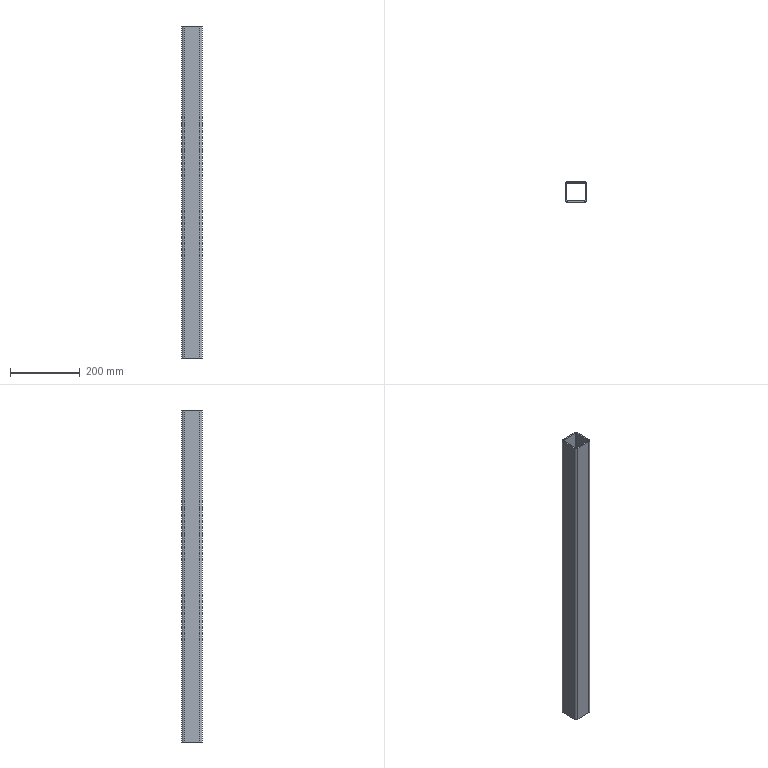Part | SolidWorks | features ICE 1, LibraryFeature 1 | 1 solid | 18 faces | box 60 x 60 x 950 mm | volume 812057 mm3 | plane 10 | cylinder 8 | commonest cylinder face diameters 8 x4 16 x4
STEP:
#1=CARTESIAN_POINT('',(22.,30.,0.));
#2=VERTEX_POINT('',#1);
#3=CARTESIAN_POINT('',(-22.,30.,0.));
#4=VERTEX_POINT('',#3);
#5=CARTESIAN_POINT('',(0.,30.,0.));
#6=DIRECTION('',(-1.,0.,0.));
#7=VECTOR('',#6,1000.);
#8=LINE('',#5,#7);
#9=EDGE_CURVE('',#2,#4,#8,.T.);
#10=ORIENTED_EDGE('',*,*,#9,.T.);
#11=CARTESIAN_POINT('',(-22.,30.,950.));
#12=VERTEX_POINT('',#11);
#13=CARTESIAN_POINT('',(-22.,30.,950.));
#14=DIRECTION('',(0.,0.,-1.));
#15=VECTOR('',#14,1000.);
#16=LINE('',#13,#15);
#17=EDGE_CURVE('',#12,#4,#16,.T.);
#18=ORIENTED_EDGE('',*,*,#17,.F.);
#19=CARTESIAN_POINT('',(22.,30.,950.));
#20=VERTEX_POINT('',#19);
#21=CARTESIAN_POINT('',(0.,30.,950.));
#22=DIRECTION('',(-1.,0.,0.));
#23=VECTOR('',#22,1000.);
#24=LINE('',#21,#23);
#25=EDGE_CURVE('',#20,#12,#24,.T.);
#26=ORIENTED_EDGE('',*,*,#25,.F.);
#27=CARTESIAN_POINT('',(22.,30.,950.));
#28=DIRECTION('',(0.,0.,-1.));
#29=VECTOR('',#28,1000.);
#30=LINE('',#27,#29);
#31=EDGE_CURVE('',#20,#2,#30,.T.);
#32=ORIENTED_EDGE('',*,*,#31,.T.);
#33=EDGE_LOOP('',(#10,#18,#26,#32));
#34=FACE_OUTER_BOUND('',#33,.T.);
#35=CARTESIAN_POINT('',(0.,30.,950.));
#36=DIRECTION('',(0.,-1.,0.));
#37=DIRECTION('',(0.,0.,-1.));
#38=AXIS2_PLACEMENT_3D('',#35,#36,#37);
#39=PLANE('',#38);
#40=ADVANCED_FACE('',(#34),#39,.F.);
#41=CARTESIAN_POINT('',(-30.,22.,0.));
#42=VERTEX_POINT('',#41);
#43=CARTESIAN_POINT('',(-22.,22.,0.));
#44=DIRECTION('',(0.,0.,1.));
#45=DIRECTION('',(1.,0.,0.));
#46=AXIS2_PLACEMENT_3D('',#43,#44,#45);
#47=CIRCLE('',#46,8.);
#48=EDGE_CURVE('',#4,#42,#47,.T.);
#49=ORIENTED_EDGE('',*,*,#48,.T.);
#50=CARTESIAN_POINT('',(-30.,22.,950.));
#51=VERTEX_POINT('',#50);
#52=CARTESIAN_POINT('',(-30.,22.,950.));
#53=DIRECTION('',(0.,0.,-1.));
#54=VECTOR('',#53,1000.);
#55=LINE('',#52,#54);
#56=EDGE_CURVE('',#51,#42,#55,.T.);
#57=ORIENTED_EDGE('',*,*,#56,.F.);
#58=CARTESIAN_POINT('',(-22.,22.,950.));
#59=DIRECTION('',(0.,0.,1.));
#60=DIRECTION('',(1.,0.,0.));
#61=AXIS2_PLACEMENT_3D('',#58,#59,#60);
#62=CIRCLE('',#61,8.);
#63=EDGE_CURVE('',#12,#51,#62,.T.);
#64=ORIENTED_EDGE('',*,*,#63,.F.);
#65=ORIENTED_EDGE('',*,*,#17,.T.);
#66=EDGE_LOOP('',(#49,#57,#64,#65));
#67=FACE_OUTER_BOUND('',#66,.T.);
#68=CARTESIAN_POINT('',(-22.,22.,950.));
#69=DIRECTION('',(0.,0.,-1.));
#70=DIRECTION('',(-1.,0.,0.));
#71=AXIS2_PLACEMENT_3D('',#68,#69,#70);
#72=CYLINDRICAL_SURFACE('',#71,8.);
#73=ADVANCED_FACE('',(#67),#72,.T.);
#74=CARTESIAN_POINT('',(-30.,-22.,0.));
#75=VERTEX_POINT('',#74);
#76=CARTESIAN_POINT('',(-30.,0.,0.));
#77=DIRECTION('',(0.,1.,0.));
#78=VECTOR('',#77,1000.);
#79=LINE('',#76,#78);
#80=EDGE_CURVE('',#75,#42,#79,.T.);
#81=ORIENTED_EDGE('',*,*,#80,.F.);
#82=CARTESIAN_POINT('',(-30.,-22.,950.));
#83=VERTEX_POINT('',#82);
#84=CARTESIAN_POINT('',(-30.,-22.,950.));
#85=DIRECTION('',(0.,0.,-1.));
#86=VECTOR('',#85,1000.);
#87=LINE('',#84,#86);
#88=EDGE_CURVE('',#83,#75,#87,.T.);
#89=ORIENTED_EDGE('',*,*,#88,.F.);
#90=CARTESIAN_POINT('',(-30.,0.,950.));
#91=DIRECTION('',(0.,1.,0.));
#92=VECTOR('',#91,1000.);
#93=LINE('',#90,#92);
#94=EDGE_CURVE('',#83,#51,#93,.T.);
#95=ORIENTED_EDGE('',*,*,#94,.T.);
#96=ORIENTED_EDGE('',*,*,#56,.T.);
#97=EDGE_LOOP('',(#81,#89,#95,#96));
#98=FACE_OUTER_BOUND('',#97,.T.);
#99=CARTESIAN_POINT('',(-30.,0.,950.));
#100=DIRECTION('',(-1.,0.,0.));
#101=DIRECTION('',(0.,0.,1.));
#102=AXIS2_PLACEMENT_3D('',#99,#100,#101);
#103=PLANE('',#102);
#104=ADVANCED_FACE('',(#98),#103,.T.);
#105=CARTESIAN_POINT('',(-22.,-30.,0.));
#106=VERTEX_POINT('',#105);
#107=CARTESIAN_POINT('',(-22.,-22.,0.));
#108=DIRECTION('',(0.,0.,1.));
#109=DIRECTION('',(1.,0.,0.));
#110=AXIS2_PLACEMENT_3D('',#107,#108,#109);
#111=CIRCLE('',#110,8.);
#112=EDGE_CURVE('',#75,#106,#111,.T.);
#113=ORIENTED_EDGE('',*,*,#112,.T.);
#114=CARTESIAN_POINT('',(-22.,-30.,950.));
#115=VERTEX_POINT('',#114);
#116=CARTESIAN_POINT('',(-22.,-30.,950.));
#117=DIRECTION('',(0.,0.,-1.));
#118=VECTOR('',#117,1000.);
#119=LINE('',#116,#118);
#120=EDGE_CURVE('',#115,#106,#119,.T.);
#121=ORIENTED_EDGE('',*,*,#120,.F.);
#122=CARTESIAN_POINT('',(-22.,-22.,950.));
#123=DIRECTION('',(0.,0.,1.));
#124=DIRECTION('',(1.,0.,0.));
#125=AXIS2_PLACEMENT_3D('',#122,#123,#124);
#126=CIRCLE('',#125,8.);
#127=EDGE_CURVE('',#83,#115,#126,.T.);
#128=ORIENTED_EDGE('',*,*,#127,.F.);
#129=ORIENTED_EDGE('',*,*,#88,.T.);
#130=EDGE_LOOP('',(#113,#121,#128,#129));
#131=FACE_OUTER_BOUND('',#130,.T.);
#132=CARTESIAN_POINT('',(-22.,-22.,950.));
#133=DIRECTION('',(0.,0.,-1.));
#134=DIRECTION('',(-1.,0.,0.));
#135=AXIS2_PLACEMENT_3D('',#132,#133,#134);
#136=CYLINDRICAL_SURFACE('',#135,8.);
#137=ADVANCED_FACE('',(#131),#136,.T.);
#138=CARTESIAN_POINT('',(22.,-30.,0.));
#139=VERTEX_POINT('',#138);
#140=CARTESIAN_POINT('',(0.,-30.,0.));
#141=DIRECTION('',(1.,0.,0.));
#142=VECTOR('',#141,1000.);
#143=LINE('',#140,#142);
#144=EDGE_CURVE('',#106,#139,#143,.T.);
#145=ORIENTED_EDGE('',*,*,#144,.T.);
#146=CARTESIAN_POINT('',(22.,-30.,950.));
#147=VERTEX_POINT('',#146);
#148=CARTESIAN_POINT('',(22.,-30.,950.));
#149=DIRECTION('',(0.,0.,-1.));
#150=VECTOR('',#149,1000.);
#151=LINE('',#148,#150);
#152=EDGE_CURVE('',#147,#139,#151,.T.);
#153=ORIENTED_EDGE('',*,*,#152,.F.);
#154=CARTESIAN_POINT('',(0.,-30.,950.));
#155=DIRECTION('',(1.,0.,0.));
#156=VECTOR('',#155,1000.);
#157=LINE('',#154,#156);
#158=EDGE_CURVE('',#115,#147,#157,.T.);
#159=ORIENTED_EDGE('',*,*,#158,.F.);
#160=ORIENTED_EDGE('',*,*,#120,.T.);
#161=EDGE_LOOP('',(#145,#153,#159,#160));
#162=FACE_OUTER_BOUND('',#161,.T.);
#163=CARTESIAN_POINT('',(0.,-30.,950.));
#164=DIRECTION('',(0.,1.,0.));
#165=DIRECTION('',(0.,0.,1.));
#166=AXIS2_PLACEMENT_3D('',#163,#164,#165);
#167=PLANE('',#166);
#168=ADVANCED_FACE('',(#162),#167,.F.);
#169=CARTESIAN_POINT('',(30.,-22.,0.));
#170=VERTEX_POINT('',#169);
#171=CARTESIAN_POINT('',(22.,-22.,0.));
#172=DIRECTION('',(0.,0.,1.));
#173=DIRECTION('',(1.,0.,0.));
#174=AXIS2_PLACEMENT_3D('',#171,#172,#173);
#175=CIRCLE('',#174,8.);
#176=EDGE_CURVE('',#139,#170,#175,.T.);
#177=ORIENTED_EDGE('',*,*,#176,.T.);
#178=CARTESIAN_POINT('',(30.,-22.,950.));
#179=VERTEX_POINT('',#178);
#180=CARTESIAN_POINT('',(30.,-22.,950.));
#181=DIRECTION('',(0.,0.,-1.));
#182=VECTOR('',#181,1000.);
#183=LINE('',#180,#182);
#184=EDGE_CURVE('',#179,#170,#183,.T.);
#185=ORIENTED_EDGE('',*,*,#184,.F.);
#186=CARTESIAN_POINT('',(22.,-22.,950.));
#187=DIRECTION('',(0.,0.,1.));
#188=DIRECTION('',(1.,0.,0.));
#189=AXIS2_PLACEMENT_3D('',#186,#187,#188);
#190=CIRCLE('',#189,8.);
#191=EDGE_CURVE('',#147,#179,#190,.T.);
#192=ORIENTED_EDGE('',*,*,#191,.F.);
#193=ORIENTED_EDGE('',*,*,#152,.T.);
#194=EDGE_LOOP('',(#177,#185,#192,#193));
#195=FACE_OUTER_BOUND('',#194,.T.);
#196=CARTESIAN_POINT('',(22.,-22.,950.));
#197=DIRECTION('',(0.,0.,-1.));
#198=DIRECTION('',(-1.,0.,0.));
#199=AXIS2_PLACEMENT_3D('',#196,#197,#198);
#200=CYLINDRICAL_SURFACE('',#199,8.);
#201=ADVANCED_FACE('',(#195),#200,.T.);
#202=CARTESIAN_POINT('',(30.,22.,0.));
#203=VERTEX_POINT('',#202);
#204=CARTESIAN_POINT('',(30.,0.,0.));
#205=DIRECTION('',(0.,-1.,0.));
#206=VECTOR('',#205,1000.);
#207=LINE('',#204,#206);
#208=EDGE_CURVE('',#203,#170,#207,.T.);
#209=ORIENTED_EDGE('',*,*,#208,.F.);
#210=CARTESIAN_POINT('',(30.,22.,950.));
#211=VERTEX_POINT('',#210);
#212=CARTESIAN_POINT('',(30.,22.,950.));
#213=DIRECTION('',(0.,0.,-1.));
#214=VECTOR('',#213,1000.);
#215=LINE('',#212,#214);
#216=EDGE_CURVE('',#211,#203,#215,.T.);
#217=ORIENTED_EDGE('',*,*,#216,.F.);
#218=CARTESIAN_POINT('',(30.,0.,950.));
#219=DIRECTION('',(0.,-1.,0.));
#220=VECTOR('',#219,1000.);
#221=LINE('',#218,#220);
#222=EDGE_CURVE('',#211,#179,#221,.T.);
#223=ORIENTED_EDGE('',*,*,#222,.T.);
#224=ORIENTED_EDGE('',*,*,#184,.T.);
#225=EDGE_LOOP('',(#209,#217,#223,#224));
#226=FACE_OUTER_BOUND('',#225,.T.);
#227=CARTESIAN_POINT('',(30.,0.,950.));
#228=DIRECTION('',(1.,0.,0.));
#229=DIRECTION('',(0.,0.,-1.));
#230=AXIS2_PLACEMENT_3D('',#227,#228,#229);
#231=PLANE('',#230);
#232=ADVANCED_FACE('',(#226),#231,.T.);
#233=CARTESIAN_POINT('',(-26.,-22.,0.));
#234=VERTEX_POINT('',#233);
#235=CARTESIAN_POINT('',(-22.,-26.,0.));
#236=VERTEX_POINT('',#235);
#237=CARTESIAN_POINT('',(-22.,-22.,0.));
#238=DIRECTION('',(0.,0.,1.));
#239=DIRECTION('',(1.,0.,0.));
#240=AXIS2_PLACEMENT_3D('',#237,#238,#239);
#241=CIRCLE('',#240,4.);
#242=EDGE_CURVE('',#234,#236,#241,.T.);
#243=ORIENTED_EDGE('',*,*,#242,.F.);
#244=CARTESIAN_POINT('',(-26.,-22.,950.));
#245=VERTEX_POINT('',#244);
#246=CARTESIAN_POINT('',(-26.,-22.,950.));
#247=DIRECTION('',(0.,0.,-1.));
#248=VECTOR('',#247,1000.);
#249=LINE('',#246,#248);
#250=EDGE_CURVE('',#245,#234,#249,.T.);
#251=ORIENTED_EDGE('',*,*,#250,.F.);
#252=CARTESIAN_POINT('',(-22.,-26.,950.));
#253=VERTEX_POINT('',#252);
#254=CARTESIAN_POINT('',(-22.,-22.,950.));
#255=DIRECTION('',(0.,0.,1.));
#256=DIRECTION('',(1.,0.,0.));
#257=AXIS2_PLACEMENT_3D('',#254,#255,#256);
#258=CIRCLE('',#257,4.);
#259=EDGE_CURVE('',#245,#253,#258,.T.);
#260=ORIENTED_EDGE('',*,*,#259,.T.);
#261=CARTESIAN_POINT('',(-22.,-26.,950.));
#262=DIRECTION('',(0.,0.,-1.));
#263=VECTOR('',#262,1000.);
#264=LINE('',#261,#263);
#265=EDGE_CURVE('',#253,#236,#264,.T.);
#266=ORIENTED_EDGE('',*,*,#265,.T.);
#267=EDGE_LOOP('',(#243,#251,#260,#266));
#268=FACE_OUTER_BOUND('',#267,.T.);
#269=CARTESIAN_POINT('',(-22.,-22.,950.));
#270=DIRECTION('',(0.,0.,-1.));
#271=DIRECTION('',(-1.,0.,0.));
#272=AXIS2_PLACEMENT_3D('',#269,#270,#271);
#273=CYLINDRICAL_SURFACE('',#272,4.);
#274=ADVANCED_FACE('',(#268),#273,.F.);
#275=CARTESIAN_POINT('',(-26.,22.,0.));
#276=VERTEX_POINT('',#275);
#277=CARTESIAN_POINT('',(-26.,0.,0.));
#278=DIRECTION('',(0.,1.,0.));
#279=VECTOR('',#278,1000.);
#280=LINE('',#277,#279);
#281=EDGE_CURVE('',#234,#276,#280,.T.);
#282=ORIENTED_EDGE('',*,*,#281,.T.);
#283=CARTESIAN_POINT('',(-26.,22.,950.));
#284=VERTEX_POINT('',#283);
#285=CARTESIAN_POINT('',(-26.,22.,950.));
#286=DIRECTION('',(0.,0.,-1.));
#287=VECTOR('',#286,1000.);
#288=LINE('',#285,#287);
#289=EDGE_CURVE('',#284,#276,#288,.T.);
#290=ORIENTED_EDGE('',*,*,#289,.F.);
#291=CARTESIAN_POINT('',(-26.,0.,950.));
#292=DIRECTION('',(0.,1.,0.));
#293=VECTOR('',#292,1000.);
#294=LINE('',#291,#293);
#295=EDGE_CURVE('',#245,#284,#294,.T.);
#296=ORIENTED_EDGE('',*,*,#295,.F.);
#297=ORIENTED_EDGE('',*,*,#250,.T.);
#298=EDGE_LOOP('',(#282,#290,#296,#297));
#299=FACE_OUTER_BOUND('',#298,.T.);
#300=CARTESIAN_POINT('',(-26.,0.,950.));
#301=DIRECTION('',(-1.,0.,0.));
#302=DIRECTION('',(0.,0.,1.));
#303=AXIS2_PLACEMENT_3D('',#300,#301,#302);
#304=PLANE('',#303);
#305=ADVANCED_FACE('',(#299),#304,.F.);
#306=CARTESIAN_POINT('',(-22.,26.,0.));
#307=VERTEX_POINT('',#306);
#308=CARTESIAN_POINT('',(-22.,22.,0.));
#309=DIRECTION('',(0.,0.,1.));
#310=DIRECTION('',(1.,0.,0.));
#311=AXIS2_PLACEMENT_3D('',#308,#309,#310);
#312=CIRCLE('',#311,4.);
#313=EDGE_CURVE('',#307,#276,#312,.T.);
#314=ORIENTED_EDGE('',*,*,#313,.F.);
#315=CARTESIAN_POINT('',(-22.,26.,950.));
#316=VERTEX_POINT('',#315);
#317=CARTESIAN_POINT('',(-22.,26.,950.));
#318=DIRECTION('',(0.,0.,-1.));
#319=VECTOR('',#318,1000.);
#320=LINE('',#317,#319);
#321=EDGE_CURVE('',#316,#307,#320,.T.);
#322=ORIENTED_EDGE('',*,*,#321,.F.);
#323=CARTESIAN_POINT('',(-22.,22.,950.));
#324=DIRECTION('',(0.,0.,1.));
#325=DIRECTION('',(1.,0.,0.));
#326=AXIS2_PLACEMENT_3D('',#323,#324,#325);
#327=CIRCLE('',#326,4.);
#328=EDGE_CURVE('',#316,#284,#327,.T.);
#329=ORIENTED_EDGE('',*,*,#328,.T.);
#330=ORIENTED_EDGE('',*,*,#289,.T.);
#331=EDGE_LOOP('',(#314,#322,#329,#330));
#332=FACE_OUTER_BOUND('',#331,.T.);
#333=CARTESIAN_POINT('',(-22.,22.,950.));
#334=DIRECTION('',(0.,0.,-1.));
#335=DIRECTION('',(-1.,0.,0.));
#336=AXIS2_PLACEMENT_3D('',#333,#334,#335);
#337=CYLINDRICAL_SURFACE('',#336,4.);
#338=ADVANCED_FACE('',(#332),#337,.F.);
#339=CARTESIAN_POINT('',(22.,26.,0.));
#340=VERTEX_POINT('',#339);
#341=CARTESIAN_POINT('',(0.,26.,0.));
#342=DIRECTION('',(-1.,0.,0.));
#343=VECTOR('',#342,1000.);
#344=LINE('',#341,#343);
#345=EDGE_CURVE('',#340,#307,#344,.T.);
#346=ORIENTED_EDGE('',*,*,#345,.F.);
#347=CARTESIAN_POINT('',(22.,26.,950.));
#348=VERTEX_POINT('',#347);
#349=CARTESIAN_POINT('',(22.,26.,950.));
#350=DIRECTION('',(0.,0.,-1.));
#351=VECTOR('',#350,1000.);
#352=LINE('',#349,#351);
#353=EDGE_CURVE('',#348,#340,#352,.T.);
#354=ORIENTED_EDGE('',*,*,#353,.F.);
#355=CARTESIAN_POINT('',(0.,26.,950.));
#356=DIRECTION('',(-1.,0.,0.));
#357=VECTOR('',#356,1000.);
#358=LINE('',#355,#357);
#359=EDGE_CURVE('',#348,#316,#358,.T.);
#360=ORIENTED_EDGE('',*,*,#359,.T.);
#361=ORIENTED_EDGE('',*,*,#321,.T.);
#362=EDGE_LOOP('',(#346,#354,#360,#361));
#363=FACE_OUTER_BOUND('',#362,.T.);
#364=CARTESIAN_POINT('',(0.,26.,950.));
#365=DIRECTION('',(0.,-1.,0.));
#366=DIRECTION('',(0.,0.,-1.));
#367=AXIS2_PLACEMENT_3D('',#364,#365,#366);
#368=PLANE('',#367);
#369=ADVANCED_FACE('',(#363),#368,.T.);
#370=CARTESIAN_POINT('',(26.,22.,0.));
#371=VERTEX_POINT('',#370);
#372=CARTESIAN_POINT('',(22.,22.,0.));
#373=DIRECTION('',(0.,0.,1.));
#374=DIRECTION('',(1.,0.,0.));
#375=AXIS2_PLACEMENT_3D('',#372,#373,#374);
#376=CIRCLE('',#375,4.);
#377=EDGE_CURVE('',#371,#340,#376,.T.);
#378=ORIENTED_EDGE('',*,*,#377,.F.);
#379=CARTESIAN_POINT('',(26.,22.,950.));
#380=VERTEX_POINT('',#379);
#381=CARTESIAN_POINT('',(26.,22.,950.));
#382=DIRECTION('',(0.,0.,-1.));
#383=VECTOR('',#382,1000.);
#384=LINE('',#381,#383);
#385=EDGE_CURVE('',#380,#371,#384,.T.);
#386=ORIENTED_EDGE('',*,*,#385,.F.);
#387=CARTESIAN_POINT('',(22.,22.,950.));
#388=DIRECTION('',(0.,0.,1.));
#389=DIRECTION('',(1.,0.,0.));
#390=AXIS2_PLACEMENT_3D('',#387,#388,#389);
#391=CIRCLE('',#390,4.);
#392=EDGE_CURVE('',#380,#348,#391,.T.);
#393=ORIENTED_EDGE('',*,*,#392,.T.);
#394=ORIENTED_EDGE('',*,*,#353,.T.);
#395=EDGE_LOOP('',(#378,#386,#393,#394));
#396=FACE_OUTER_BOUND('',#395,.T.);
#397=CARTESIAN_POINT('',(22.,22.,950.));
#398=DIRECTION('',(0.,0.,-1.));
#399=DIRECTION('',(-1.,0.,0.));
#400=AXIS2_PLACEMENT_3D('',#397,#398,#399);
#401=CYLINDRICAL_SURFACE('',#400,4.);
#402=ADVANCED_FACE('',(#396),#401,.F.);
#403=CARTESIAN_POINT('',(26.,-22.,0.));
#404=VERTEX_POINT('',#403);
#405=CARTESIAN_POINT('',(26.,0.,0.));
#406=DIRECTION('',(0.,-1.,0.));
#407=VECTOR('',#406,1000.);
#408=LINE('',#405,#407);
#409=EDGE_CURVE('',#371,#404,#408,.T.);
#410=ORIENTED_EDGE('',*,*,#409,.T.);
#411=CARTESIAN_POINT('',(26.,-22.,950.));
#412=VERTEX_POINT('',#411);
#413=CARTESIAN_POINT('',(26.,-22.,950.));
#414=DIRECTION('',(0.,0.,-1.));
#415=VECTOR('',#414,1000.);
#416=LINE('',#413,#415);
#417=EDGE_CURVE('',#412,#404,#416,.T.);
#418=ORIENTED_EDGE('',*,*,#417,.F.);
#419=CARTESIAN_POINT('',(26.,0.,950.));
#420=DIRECTION('',(0.,-1.,0.));
#421=VECTOR('',#420,1000.);
#422=LINE('',#419,#421);
#423=EDGE_CURVE('',#380,#412,#422,.T.);
#424=ORIENTED_EDGE('',*,*,#423,.F.);
#425=ORIENTED_EDGE('',*,*,#385,.T.);
#426=EDGE_LOOP('',(#410,#418,#424,#425));
#427=FACE_OUTER_BOUND('',#426,.T.);
#428=CARTESIAN_POINT('',(26.,0.,950.));
#429=DIRECTION('',(1.,0.,0.));
#430=DIRECTION('',(0.,0.,-1.));
#431=AXIS2_PLACEMENT_3D('',#428,#429,#430);
#432=PLANE('',#431);
#433=ADVANCED_FACE('',(#427),#432,.F.);
#434=CARTESIAN_POINT('',(22.,-26.,0.));
#435=VERTEX_POINT('',#434);
#436=CARTESIAN_POINT('',(22.,-22.,0.));
#437=DIRECTION('',(0.,0.,1.));
#438=DIRECTION('',(1.,0.,0.));
#439=AXIS2_PLACEMENT_3D('',#436,#437,#438);
#440=CIRCLE('',#439,4.);
#441=EDGE_CURVE('',#435,#404,#440,.T.);
#442=ORIENTED_EDGE('',*,*,#441,.F.);
#443=CARTESIAN_POINT('',(22.,-26.,950.));
#444=VERTEX_POINT('',#443);
#445=CARTESIAN_POINT('',(22.,-26.,950.));
#446=DIRECTION('',(0.,0.,-1.));
#447=VECTOR('',#446,1000.);
#448=LINE('',#445,#447);
#449=EDGE_CURVE('',#444,#435,#448,.T.);
#450=ORIENTED_EDGE('',*,*,#449,.F.);
#451=CARTESIAN_POINT('',(22.,-22.,950.));
#452=DIRECTION('',(0.,0.,1.));
#453=DIRECTION('',(1.,0.,0.));
#454=AXIS2_PLACEMENT_3D('',#451,#452,#453);
#455=CIRCLE('',#454,4.);
#456=EDGE_CURVE('',#444,#412,#455,.T.);
#457=ORIENTED_EDGE('',*,*,#456,.T.);
#458=ORIENTED_EDGE('',*,*,#417,.T.);
#459=EDGE_LOOP('',(#442,#450,#457,#458));
#460=FACE_OUTER_BOUND('',#459,.T.);
#461=CARTESIAN_POINT('',(22.,-22.,950.));
#462=DIRECTION('',(0.,0.,-1.));
#463=DIRECTION('',(-1.,0.,0.));
#464=AXIS2_PLACEMENT_3D('',#461,#462,#463);
#465=CYLINDRICAL_SURFACE('',#464,4.);
#466=ADVANCED_FACE('',(#460),#465,.F.);
#467=CARTESIAN_POINT('',(0.,-26.,0.));
#468=DIRECTION('',(1.,0.,0.));
#469=VECTOR('',#468,1000.);
#470=LINE('',#467,#469);
#471=EDGE_CURVE('',#236,#435,#470,.T.);
#472=ORIENTED_EDGE('',*,*,#471,.F.);
#473=ORIENTED_EDGE('',*,*,#265,.F.);
#474=CARTESIAN_POINT('',(0.,-26.,950.));
#475=DIRECTION('',(1.,0.,0.));
#476=VECTOR('',#475,1000.);
#477=LINE('',#474,#476);
#478=EDGE_CURVE('',#253,#444,#477,.T.);
#479=ORIENTED_EDGE('',*,*,#478,.T.);
#480=ORIENTED_EDGE('',*,*,#449,.T.);
#481=EDGE_LOOP('',(#472,#473,#479,#480));
#482=FACE_OUTER_BOUND('',#481,.T.);
#483=CARTESIAN_POINT('',(0.,-26.,950.));
#484=DIRECTION('',(0.,1.,0.));
#485=DIRECTION('',(0.,0.,1.));
#486=AXIS2_PLACEMENT_3D('',#483,#484,#485);
#487=PLANE('',#486);
#488=ADVANCED_FACE('',(#482),#487,.T.);
#489=CARTESIAN_POINT('',(22.,22.,0.));
#490=DIRECTION('',(0.,0.,1.));
#491=DIRECTION('',(1.,0.,0.));
#492=AXIS2_PLACEMENT_3D('',#489,#490,#491);
#493=CIRCLE('',#492,8.);
#494=EDGE_CURVE('',#203,#2,#493,.T.);
#495=ORIENTED_EDGE('',*,*,#494,.T.);
#496=ORIENTED_EDGE('',*,*,#31,.F.);
#497=CARTESIAN_POINT('',(22.,22.,950.));
#498=DIRECTION('',(0.,0.,1.));
#499=DIRECTION('',(1.,0.,0.));
#500=AXIS2_PLACEMENT_3D('',#497,#498,#499);
#501=CIRCLE('',#500,8.);
#502=EDGE_CURVE('',#211,#20,#501,.T.);
#503=ORIENTED_EDGE('',*,*,#502,.F.);
#504=ORIENTED_EDGE('',*,*,#216,.T.);
#505=EDGE_LOOP('',(#495,#496,#503,#504));
#506=FACE_OUTER_BOUND('',#505,.T.);
#507=CARTESIAN_POINT('',(22.,22.,950.));
#508=DIRECTION('',(0.,0.,-1.));
#509=DIRECTION('',(-1.,0.,0.));
#510=AXIS2_PLACEMENT_3D('',#507,#508,#509);
#511=CYLINDRICAL_SURFACE('',#510,8.);
#512=ADVANCED_FACE('',(#506),#511,.T.);
#513=ORIENTED_EDGE('',*,*,#259,.F.);
#514=ORIENTED_EDGE('',*,*,#295,.T.);
#515=ORIENTED_EDGE('',*,*,#328,.F.);
#516=ORIENTED_EDGE('',*,*,#359,.F.);
#517=ORIENTED_EDGE('',*,*,#392,.F.);
#518=ORIENTED_EDGE('',*,*,#423,.T.);
#519=ORIENTED_EDGE('',*,*,#456,.F.);
#520=ORIENTED_EDGE('',*,*,#478,.F.);
#521=EDGE_LOOP('',(#513,#514,#515,#516,#517,#518,#519,#520));
#522=FACE_BOUND('',#521,.T.);
#523=ORIENTED_EDGE('',*,*,#25,.T.);
#524=ORIENTED_EDGE('',*,*,#63,.T.);
#525=ORIENTED_EDGE('',*,*,#94,.F.);
#526=ORIENTED_EDGE('',*,*,#127,.T.);
#527=ORIENTED_EDGE('',*,*,#158,.T.);
#528=ORIENTED_EDGE('',*,*,#191,.T.);
#529=ORIENTED_EDGE('',*,*,#222,.F.);
#530=ORIENTED_EDGE('',*,*,#502,.T.);
#531=EDGE_LOOP('',(#523,#524,#525,#526,#527,#528,#529,#530));
#532=FACE_OUTER_BOUND('',#531,.T.);
#533=CARTESIAN_POINT('',(0.,0.,950.));
#534=DIRECTION('',(0.,0.,1.));
#535=DIRECTION('',(1.,0.,0.));
#536=AXIS2_PLACEMENT_3D('',#533,#534,#535);
#537=PLANE('',#536);
#538=ADVANCED_FACE('',(#522,#532),#537,.T.);
#539=ORIENTED_EDGE('',*,*,#242,.T.);
#540=ORIENTED_EDGE('',*,*,#471,.T.);
#541=ORIENTED_EDGE('',*,*,#441,.T.);
#542=ORIENTED_EDGE('',*,*,#409,.F.);
#543=ORIENTED_EDGE('',*,*,#377,.T.);
#544=ORIENTED_EDGE('',*,*,#345,.T.);
#545=ORIENTED_EDGE('',*,*,#313,.T.);
#546=ORIENTED_EDGE('',*,*,#281,.F.);
#547=EDGE_LOOP('',(#539,#540,#541,#542,#543,#544,#545,#546));
#548=FACE_BOUND('',#547,.T.);
#549=ORIENTED_EDGE('',*,*,#9,.F.);
#550=ORIENTED_EDGE('',*,*,#494,.F.);
#551=ORIENTED_EDGE('',*,*,#208,.T.);
#552=ORIENTED_EDGE('',*,*,#176,.F.);
#553=ORIENTED_EDGE('',*,*,#144,.F.);
#554=ORIENTED_EDGE('',*,*,#112,.F.);
#555=ORIENTED_EDGE('',*,*,#80,.T.);
#556=ORIENTED_EDGE('',*,*,#48,.F.);
#557=EDGE_LOOP('',(#549,#550,#551,#552,#553,#554,#555,#556));
#558=FACE_OUTER_BOUND('',#557,.T.);
#559=CARTESIAN_POINT('',(0.,0.,0.));
#560=DIRECTION('',(0.,0.,1.));
#561=DIRECTION('',(1.,0.,0.));
#562=AXIS2_PLACEMENT_3D('',#559,#560,#561);
#563=PLANE('',#562);
#564=ADVANCED_FACE('',(#548,#558),#563,.F.);
#565=CLOSED_SHELL('',(#40,#73,#104,#137,#168,#201,#232,#274,#305,#338,#369,#402,#433,#466,#488,#512,#538,#564));
#566=MANIFOLD_SOLID_BREP('',#565);
#567=CARTESIAN_POINT('',(0.,0.,0.));
#568=DIRECTION('',(0.,0.,1.));
#569=DIRECTION('',(1.,0.,0.));
#570=AXIS2_PLACEMENT_3D('',#567,#568,#569);
#571=(LENGTH_UNIT()NAMED_UNIT(*)SI_UNIT(.MILLI.,.METRE.));
#572=UNCERTAINTY_MEASURE_WITH_UNIT(LENGTH_MEASURE(0.00001),#571,'','');
#573=(NAMED_UNIT(*)PLANE_ANGLE_UNIT()SI_UNIT($,.RADIAN.));
#574=(NAMED_UNIT(*)SI_UNIT($,.STERADIAN.)SOLID_ANGLE_UNIT());
#575=(GEOMETRIC_REPRESENTATION_CONTEXT(3)GLOBAL_UNCERTAINTY_ASSIGNED_CONTEXT((#572))GLOBAL_UNIT_ASSIGNED_CONTEXT((#571,#573,#574))REPRESENTATION_CONTEXT('',''));
#576=ADVANCED_BREP_SHAPE_REPRESENTATION('',(#566,#570),#575);